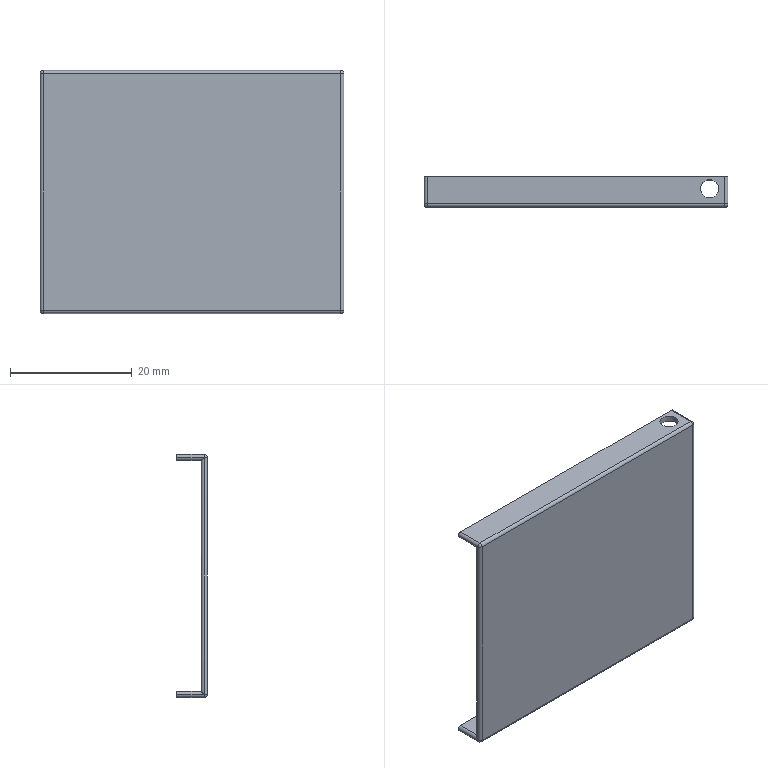Part | SolidWorks | features ICE 2, Extrusion 1, Fillet 1, MirrorPattern 1, MoveFace 1 | 1 solid | 31 faces | box 50 x 5 x 40 mm | volume 2370 mm3 | cylinder 19 | plane 8 | sphere 4 | commonest cylinder face diameters 1 x15 3 x4
STEP:
#1=CARTESIAN_POINT('',(23.5,3.,-19.));
#2=VERTEX_POINT('',#1);
#3=CARTESIAN_POINT('',(20.5,3.,-19.));
#4=VERTEX_POINT('',#3);
#5=CARTESIAN_POINT('',(22.,3.,-19.));
#6=DIRECTION('',(0.,0.,-1.));
#7=DIRECTION('',(-1.,0.,0.));
#8=AXIS2_PLACEMENT_3D('',#5,#6,#7);
#9=CIRCLE('',#8,1.5);
#10=EDGE_CURVE('',#2,#4,#9,.T.);
#11=ORIENTED_EDGE('',*,*,#10,.F.);
#12=CARTESIAN_POINT('',(23.5,3.,-20.));
#13=VERTEX_POINT('',#12);
#14=CARTESIAN_POINT('',(23.5,3.,20.));
#15=DIRECTION('',(0.,0.,-1.));
#16=VECTOR('',#15,1000.);
#17=LINE('',#14,#16);
#18=EDGE_CURVE('',#2,#13,#17,.T.);
#19=ORIENTED_EDGE('',*,*,#18,.T.);
#20=CARTESIAN_POINT('',(20.5,3.,-20.));
#21=VERTEX_POINT('',#20);
#22=CARTESIAN_POINT('',(22.,3.,-20.));
#23=DIRECTION('',(0.,0.,-1.));
#24=DIRECTION('',(-1.,0.,0.));
#25=AXIS2_PLACEMENT_3D('',#22,#23,#24);
#26=CIRCLE('',#25,1.5);
#27=EDGE_CURVE('',#13,#21,#26,.T.);
#28=ORIENTED_EDGE('',*,*,#27,.T.);
#29=CARTESIAN_POINT('',(20.5,3.,20.));
#30=DIRECTION('',(0.,0.,-1.));
#31=VECTOR('',#30,1000.);
#32=LINE('',#29,#31);
#33=EDGE_CURVE('',#4,#21,#32,.T.);
#34=ORIENTED_EDGE('',*,*,#33,.F.);
#35=EDGE_LOOP('',(#11,#19,#28,#34));
#36=FACE_OUTER_BOUND('',#35,.T.);
#37=CARTESIAN_POINT('',(22.,3.,20.));
#38=DIRECTION('',(0.,0.,-1.));
#39=DIRECTION('',(-1.,0.,0.));
#40=AXIS2_PLACEMENT_3D('',#37,#38,#39);
#41=CYLINDRICAL_SURFACE('',#40,1.5);
#42=ADVANCED_FACE('',(#36),#41,.F.);
#43=CARTESIAN_POINT('',(23.5,3.,20.));
#44=VERTEX_POINT('',#43);
#45=CARTESIAN_POINT('',(20.5,3.,20.));
#46=VERTEX_POINT('',#45);
#47=CARTESIAN_POINT('',(22.,3.,20.));
#48=DIRECTION('',(0.,0.,-1.));
#49=DIRECTION('',(-1.,0.,0.));
#50=AXIS2_PLACEMENT_3D('',#47,#48,#49);
#51=CIRCLE('',#50,1.5);
#52=EDGE_CURVE('',#44,#46,#51,.T.);
#53=ORIENTED_EDGE('',*,*,#52,.F.);
#54=CARTESIAN_POINT('',(23.5,3.,19.));
#55=VERTEX_POINT('',#54);
#56=CARTESIAN_POINT('',(23.5,3.,20.));
#57=DIRECTION('',(0.,0.,-1.));
#58=VECTOR('',#57,1000.);
#59=LINE('',#56,#58);
#60=EDGE_CURVE('',#44,#55,#59,.T.);
#61=ORIENTED_EDGE('',*,*,#60,.T.);
#62=CARTESIAN_POINT('',(20.5,3.,19.));
#63=VERTEX_POINT('',#62);
#64=CARTESIAN_POINT('',(22.,3.,19.));
#65=DIRECTION('',(0.,0.,1.));
#66=DIRECTION('',(1.,0.,0.));
#67=AXIS2_PLACEMENT_3D('',#64,#65,#66);
#68=CIRCLE('',#67,1.5);
#69=EDGE_CURVE('',#63,#55,#68,.T.);
#70=ORIENTED_EDGE('',*,*,#69,.F.);
#71=CARTESIAN_POINT('',(20.5,3.,20.));
#72=DIRECTION('',(0.,0.,-1.));
#73=VECTOR('',#72,1000.);
#74=LINE('',#71,#73);
#75=EDGE_CURVE('',#46,#63,#74,.T.);
#76=ORIENTED_EDGE('',*,*,#75,.F.);
#77=EDGE_LOOP('',(#53,#61,#70,#76));
#78=FACE_OUTER_BOUND('',#77,.T.);
#79=CARTESIAN_POINT('',(22.,3.,20.));
#80=DIRECTION('',(0.,0.,-1.));
#81=DIRECTION('',(-1.,0.,0.));
#82=AXIS2_PLACEMENT_3D('',#79,#80,#81);
#83=CYLINDRICAL_SURFACE('',#82,1.5);
#84=ADVANCED_FACE('',(#78),#83,.F.);
#85=CARTESIAN_POINT('',(24.5,1.,19.));
#86=VERTEX_POINT('',#85);
#87=CARTESIAN_POINT('',(-24.5,1.,19.));
#88=VERTEX_POINT('',#87);
#89=CARTESIAN_POINT('',(-25.,1.,19.));
#90=DIRECTION('',(-1.,0.,0.));
#91=VECTOR('',#90,1000.);
#92=LINE('',#89,#91);
#93=EDGE_CURVE('',#86,#88,#92,.T.);
#94=ORIENTED_EDGE('',*,*,#93,.F.);
#95=CARTESIAN_POINT('',(24.5,1.,-19.));
#96=VERTEX_POINT('',#95);
#97=CARTESIAN_POINT('',(24.5,1.,0.));
#98=DIRECTION('',(0.,0.,-1.));
#99=VECTOR('',#98,1000.);
#100=LINE('',#97,#99);
#101=EDGE_CURVE('',#86,#96,#100,.T.);
#102=ORIENTED_EDGE('',*,*,#101,.T.);
#103=CARTESIAN_POINT('',(-24.5,1.,-19.));
#104=VERTEX_POINT('',#103);
#105=CARTESIAN_POINT('',(-25.,1.,-19.));
#106=DIRECTION('',(-1.,0.,0.));
#107=VECTOR('',#106,1000.);
#108=LINE('',#105,#107);
#109=EDGE_CURVE('',#96,#104,#108,.T.);
#110=ORIENTED_EDGE('',*,*,#109,.T.);
#111=CARTESIAN_POINT('',(-24.5,1.,0.));
#112=DIRECTION('',(0.,0.,1.));
#113=VECTOR('',#112,1000.);
#114=LINE('',#111,#113);
#115=EDGE_CURVE('',#104,#88,#114,.T.);
#116=ORIENTED_EDGE('',*,*,#115,.T.);
#117=EDGE_LOOP('',(#94,#102,#110,#116));
#118=FACE_OUTER_BOUND('',#117,.T.);
#119=CARTESIAN_POINT('',(0.,1.,0.));
#120=DIRECTION('',(0.,-1.,0.));
#121=DIRECTION('',(0.,0.,-1.));
#122=AXIS2_PLACEMENT_3D('',#119,#120,#121);
#123=PLANE('',#122);
#124=ADVANCED_FACE('',(#118),#123,.F.);
#125=CARTESIAN_POINT('',(22.,3.,-20.));
#126=DIRECTION('',(0.,0.,-1.));
#127=DIRECTION('',(-1.,0.,0.));
#128=AXIS2_PLACEMENT_3D('',#125,#126,#127);
#129=CIRCLE('',#128,1.5);
#130=EDGE_CURVE('',#21,#13,#129,.T.);
#131=ORIENTED_EDGE('',*,*,#130,.F.);
#132=ORIENTED_EDGE('',*,*,#27,.F.);
#133=EDGE_LOOP('',(#131,#132));
#134=FACE_BOUND('',#133,.T.);
#135=CARTESIAN_POINT('',(24.5,0.5,-20.));
#136=VERTEX_POINT('',#135);
#137=CARTESIAN_POINT('',(-24.5,0.5,-20.));
#138=VERTEX_POINT('',#137);
#139=CARTESIAN_POINT('',(-25.,0.5,-20.));
#140=DIRECTION('',(-1.,0.,0.));
#141=VECTOR('',#140,1000.);
#142=LINE('',#139,#141);
#143=EDGE_CURVE('',#136,#138,#142,.T.);
#144=ORIENTED_EDGE('',*,*,#143,.T.);
#145=CARTESIAN_POINT('',(-24.5,5.,-20.));
#146=VERTEX_POINT('',#145);
#147=CARTESIAN_POINT('',(-24.5,1.,-20.));
#148=DIRECTION('',(0.,1.,0.));
#149=VECTOR('',#148,1000.);
#150=LINE('',#147,#149);
#151=EDGE_CURVE('',#138,#146,#150,.T.);
#152=ORIENTED_EDGE('',*,*,#151,.T.);
#153=CARTESIAN_POINT('',(24.5,5.,-20.));
#154=VERTEX_POINT('',#153);
#155=CARTESIAN_POINT('',(-25.,5.,-20.));
#156=DIRECTION('',(1.,0.,0.));
#157=VECTOR('',#156,1000.);
#158=LINE('',#155,#157);
#159=EDGE_CURVE('',#146,#154,#158,.T.);
#160=ORIENTED_EDGE('',*,*,#159,.T.);
#161=CARTESIAN_POINT('',(24.5,1.,-20.));
#162=DIRECTION('',(0.,-1.,0.));
#163=VECTOR('',#162,1000.);
#164=LINE('',#161,#163);
#165=EDGE_CURVE('',#154,#136,#164,.T.);
#166=ORIENTED_EDGE('',*,*,#165,.T.);
#167=EDGE_LOOP('',(#144,#152,#160,#166));
#168=FACE_OUTER_BOUND('',#167,.T.);
#169=CARTESIAN_POINT('',(-25.,1.,-20.));
#170=DIRECTION('',(0.,0.,1.));
#171=DIRECTION('',(1.,0.,0.));
#172=AXIS2_PLACEMENT_3D('',#169,#170,#171);
#173=PLANE('',#172);
#174=ADVANCED_FACE('',(#134,#168),#173,.F.);
#175=CARTESIAN_POINT('',(22.,3.,20.));
#176=DIRECTION('',(0.,0.,-1.));
#177=DIRECTION('',(-1.,0.,0.));
#178=AXIS2_PLACEMENT_3D('',#175,#176,#177);
#179=CIRCLE('',#178,1.5);
#180=EDGE_CURVE('',#46,#44,#179,.T.);
#181=ORIENTED_EDGE('',*,*,#180,.T.);
#182=ORIENTED_EDGE('',*,*,#52,.T.);
#183=EDGE_LOOP('',(#181,#182));
#184=FACE_BOUND('',#183,.T.);
#185=CARTESIAN_POINT('',(-24.5,5.,20.));
#186=VERTEX_POINT('',#185);
#187=CARTESIAN_POINT('',(24.5,5.,20.));
#188=VERTEX_POINT('',#187);
#189=CARTESIAN_POINT('',(-25.,5.,20.));
#190=DIRECTION('',(1.,0.,0.));
#191=VECTOR('',#190,1000.);
#192=LINE('',#189,#191);
#193=EDGE_CURVE('',#186,#188,#192,.T.);
#194=ORIENTED_EDGE('',*,*,#193,.F.);
#195=CARTESIAN_POINT('',(-24.5,0.5,20.));
#196=VERTEX_POINT('',#195);
#197=CARTESIAN_POINT('',(-24.5,1.,20.));
#198=DIRECTION('',(0.,-1.,0.));
#199=VECTOR('',#198,1000.);
#200=LINE('',#197,#199);
#201=EDGE_CURVE('',#186,#196,#200,.T.);
#202=ORIENTED_EDGE('',*,*,#201,.T.);
#203=CARTESIAN_POINT('',(24.5,0.5,20.));
#204=VERTEX_POINT('',#203);
#205=CARTESIAN_POINT('',(25.,0.5,20.));
#206=DIRECTION('',(1.,0.,0.));
#207=VECTOR('',#206,1000.);
#208=LINE('',#205,#207);
#209=EDGE_CURVE('',#196,#204,#208,.T.);
#210=ORIENTED_EDGE('',*,*,#209,.T.);
#211=CARTESIAN_POINT('',(24.5,1.,20.));
#212=DIRECTION('',(0.,1.,0.));
#213=VECTOR('',#212,1000.);
#214=LINE('',#211,#213);
#215=EDGE_CURVE('',#204,#188,#214,.T.);
#216=ORIENTED_EDGE('',*,*,#215,.T.);
#217=EDGE_LOOP('',(#194,#202,#210,#216));
#218=FACE_OUTER_BOUND('',#217,.T.);
#219=CARTESIAN_POINT('',(-25.,1.,20.));
#220=DIRECTION('',(0.,0.,-1.));
#221=DIRECTION('',(-1.,0.,0.));
#222=AXIS2_PLACEMENT_3D('',#219,#220,#221);
#223=PLANE('',#222);
#224=ADVANCED_FACE('',(#184,#218),#223,.F.);
#225=CARTESIAN_POINT('',(-24.5,0.,19.5));
#226=VERTEX_POINT('',#225);
#227=CARTESIAN_POINT('',(-24.5,0.,-19.5));
#228=VERTEX_POINT('',#227);
#229=CARTESIAN_POINT('',(-24.5,0.,-20.));
#230=DIRECTION('',(0.,0.,-1.));
#231=VECTOR('',#230,1000.);
#232=LINE('',#229,#231);
#233=EDGE_CURVE('',#226,#228,#232,.T.);
#234=ORIENTED_EDGE('',*,*,#233,.T.);
#235=CARTESIAN_POINT('',(24.5,0.,-19.5));
#236=VERTEX_POINT('',#235);
#237=CARTESIAN_POINT('',(25.,0.,-19.5));
#238=DIRECTION('',(1.,0.,0.));
#239=VECTOR('',#238,1000.);
#240=LINE('',#237,#239);
#241=EDGE_CURVE('',#228,#236,#240,.T.);
#242=ORIENTED_EDGE('',*,*,#241,.T.);
#243=CARTESIAN_POINT('',(24.5,0.,19.5));
#244=VERTEX_POINT('',#243);
#245=CARTESIAN_POINT('',(24.5,0.,20.));
#246=DIRECTION('',(0.,0.,1.));
#247=VECTOR('',#246,1000.);
#248=LINE('',#245,#247);
#249=EDGE_CURVE('',#236,#244,#248,.T.);
#250=ORIENTED_EDGE('',*,*,#249,.T.);
#251=CARTESIAN_POINT('',(-25.,0.,19.5));
#252=DIRECTION('',(-1.,0.,0.));
#253=VECTOR('',#252,1000.);
#254=LINE('',#251,#253);
#255=EDGE_CURVE('',#244,#226,#254,.T.);
#256=ORIENTED_EDGE('',*,*,#255,.T.);
#257=EDGE_LOOP('',(#234,#242,#250,#256));
#258=FACE_OUTER_BOUND('',#257,.T.);
#259=CARTESIAN_POINT('',(0.,0.,0.));
#260=DIRECTION('',(0.,-1.,0.));
#261=DIRECTION('',(0.,0.,-1.));
#262=AXIS2_PLACEMENT_3D('',#259,#260,#261);
#263=PLANE('',#262);
#264=ADVANCED_FACE('',(#258),#263,.T.);
#265=CARTESIAN_POINT('',(-25.,5.,-19.5));
#266=VERTEX_POINT('',#265);
#267=CARTESIAN_POINT('',(-24.5,5.,-19.5));
#268=DIRECTION('',(0.,1.,0.));
#269=DIRECTION('',(-1.,0.,0.));
#270=AXIS2_PLACEMENT_3D('',#267,#268,#269);
#271=CIRCLE('',#270,0.5);
#272=EDGE_CURVE('',#146,#266,#271,.T.);
#273=ORIENTED_EDGE('',*,*,#272,.T.);
#274=CARTESIAN_POINT('',(-24.5,5.,-19.));
#275=VERTEX_POINT('',#274);
#276=CARTESIAN_POINT('',(-24.5,5.,-19.5));
#277=DIRECTION('',(0.,1.,0.));
#278=DIRECTION('',(-1.,0.,0.));
#279=AXIS2_PLACEMENT_3D('',#276,#277,#278);
#280=CIRCLE('',#279,0.5);
#281=EDGE_CURVE('',#266,#275,#280,.T.);
#282=ORIENTED_EDGE('',*,*,#281,.T.);
#283=CARTESIAN_POINT('',(24.5,5.,-19.));
#284=VERTEX_POINT('',#283);
#285=CARTESIAN_POINT('',(-25.,5.,-19.));
#286=DIRECTION('',(1.,0.,0.));
#287=VECTOR('',#286,1000.);
#288=LINE('',#285,#287);
#289=EDGE_CURVE('',#275,#284,#288,.T.);
#290=ORIENTED_EDGE('',*,*,#289,.T.);
#291=CARTESIAN_POINT('',(24.5,5.,-20.));
#292=DIRECTION('',(0.,0.,-1.));
#293=VECTOR('',#292,1000.);
#294=LINE('',#291,#293);
#295=EDGE_CURVE('',#284,#154,#294,.T.);
#296=ORIENTED_EDGE('',*,*,#295,.T.);
#297=ORIENTED_EDGE('',*,*,#159,.F.);
#298=EDGE_LOOP('',(#273,#282,#290,#296,#297));
#299=FACE_OUTER_BOUND('',#298,.T.);
#300=CARTESIAN_POINT('',(-25.,5.,-19.));
#301=DIRECTION('',(0.,1.,0.));
#302=DIRECTION('',(-1.,0.,0.));
#303=AXIS2_PLACEMENT_3D('',#300,#301,#302);
#304=PLANE('',#303);
#305=ADVANCED_FACE('',(#299),#304,.T.);
#306=CARTESIAN_POINT('',(22.,3.,-19.));
#307=DIRECTION('',(0.,0.,-1.));
#308=DIRECTION('',(-1.,0.,0.));
#309=AXIS2_PLACEMENT_3D('',#306,#307,#308);
#310=CIRCLE('',#309,1.5);
#311=EDGE_CURVE('',#4,#2,#310,.T.);
#312=ORIENTED_EDGE('',*,*,#311,.T.);
#313=ORIENTED_EDGE('',*,*,#10,.T.);
#314=EDGE_LOOP('',(#312,#313));
#315=FACE_BOUND('',#314,.T.);
#316=ORIENTED_EDGE('',*,*,#109,.F.);
#317=CARTESIAN_POINT('',(24.5,0.,-19.));
#318=DIRECTION('',(0.,1.,0.));
#319=VECTOR('',#318,1000.);
#320=LINE('',#317,#319);
#321=EDGE_CURVE('',#96,#284,#320,.T.);
#322=ORIENTED_EDGE('',*,*,#321,.T.);
#323=ORIENTED_EDGE('',*,*,#289,.F.);
#324=CARTESIAN_POINT('',(-24.5,0.,-19.));
#325=DIRECTION('',(0.,-1.,0.));
#326=VECTOR('',#325,1000.);
#327=LINE('',#324,#326);
#328=EDGE_CURVE('',#275,#104,#327,.T.);
#329=ORIENTED_EDGE('',*,*,#328,.T.);
#330=EDGE_LOOP('',(#316,#322,#323,#329));
#331=FACE_OUTER_BOUND('',#330,.T.);
#332=CARTESIAN_POINT('',(0.,0.,-19.));
#333=DIRECTION('',(0.,0.,-1.));
#334=DIRECTION('',(-1.,0.,0.));
#335=AXIS2_PLACEMENT_3D('',#332,#333,#334);
#336=PLANE('',#335);
#337=ADVANCED_FACE('',(#315,#331),#336,.F.);
#338=CARTESIAN_POINT('',(-24.5,5.,19.));
#339=VERTEX_POINT('',#338);
#340=CARTESIAN_POINT('',(24.5,5.,19.));
#341=VERTEX_POINT('',#340);
#342=CARTESIAN_POINT('',(-25.,5.,19.));
#343=DIRECTION('',(1.,0.,0.));
#344=VECTOR('',#343,1000.);
#345=LINE('',#342,#344);
#346=EDGE_CURVE('',#339,#341,#345,.T.);
#347=ORIENTED_EDGE('',*,*,#346,.F.);
#348=CARTESIAN_POINT('',(-25.,5.,19.5));
#349=VERTEX_POINT('',#348);
#350=CARTESIAN_POINT('',(-24.5,5.,19.5));
#351=DIRECTION('',(0.,1.,0.));
#352=DIRECTION('',(1.,0.,0.));
#353=AXIS2_PLACEMENT_3D('',#350,#351,#352);
#354=CIRCLE('',#353,0.5);
#355=EDGE_CURVE('',#339,#349,#354,.T.);
#356=ORIENTED_EDGE('',*,*,#355,.T.);
#357=CARTESIAN_POINT('',(-24.5,5.,19.5));
#358=DIRECTION('',(0.,1.,0.));
#359=DIRECTION('',(1.,0.,0.));
#360=AXIS2_PLACEMENT_3D('',#357,#358,#359);
#361=CIRCLE('',#360,0.5);
#362=EDGE_CURVE('',#349,#186,#361,.T.);
#363=ORIENTED_EDGE('',*,*,#362,.T.);
#364=ORIENTED_EDGE('',*,*,#193,.T.);
#365=CARTESIAN_POINT('',(25.,5.,19.5));
#366=VERTEX_POINT('',#365);
#367=CARTESIAN_POINT('',(24.5,5.,19.5));
#368=DIRECTION('',(0.,1.,0.));
#369=DIRECTION('',(1.,0.,0.));
#370=AXIS2_PLACEMENT_3D('',#367,#368,#369);
#371=CIRCLE('',#370,0.5);
#372=EDGE_CURVE('',#188,#366,#371,.T.);
#373=ORIENTED_EDGE('',*,*,#372,.T.);
#374=CARTESIAN_POINT('',(24.5,5.,19.5));
#375=DIRECTION('',(0.,1.,0.));
#376=DIRECTION('',(1.,0.,0.));
#377=AXIS2_PLACEMENT_3D('',#374,#375,#376);
#378=CIRCLE('',#377,0.5);
#379=EDGE_CURVE('',#366,#341,#378,.T.);
#380=ORIENTED_EDGE('',*,*,#379,.T.);
#381=EDGE_LOOP('',(#347,#356,#363,#364,#373,#380));
#382=FACE_OUTER_BOUND('',#381,.T.);
#383=CARTESIAN_POINT('',(-25.,5.,19.));
#384=DIRECTION('',(0.,-1.,0.));
#385=DIRECTION('',(1.,0.,0.));
#386=AXIS2_PLACEMENT_3D('',#383,#384,#385);
#387=PLANE('',#386);
#388=ADVANCED_FACE('',(#382),#387,.F.);
#389=ORIENTED_EDGE('',*,*,#69,.T.);
#390=CARTESIAN_POINT('',(22.,3.,19.));
#391=DIRECTION('',(0.,0.,1.));
#392=DIRECTION('',(1.,0.,0.));
#393=AXIS2_PLACEMENT_3D('',#390,#391,#392);
#394=CIRCLE('',#393,1.5);
#395=EDGE_CURVE('',#55,#63,#394,.T.);
#396=ORIENTED_EDGE('',*,*,#395,.T.);
#397=EDGE_LOOP('',(#389,#396));
#398=FACE_BOUND('',#397,.T.);
#399=ORIENTED_EDGE('',*,*,#346,.T.);
#400=CARTESIAN_POINT('',(24.5,0.,19.));
#401=DIRECTION('',(0.,-1.,0.));
#402=VECTOR('',#401,1000.);
#403=LINE('',#400,#402);
#404=EDGE_CURVE('',#341,#86,#403,.T.);
#405=ORIENTED_EDGE('',*,*,#404,.T.);
#406=ORIENTED_EDGE('',*,*,#93,.T.);
#407=CARTESIAN_POINT('',(-24.5,0.,19.));
#408=DIRECTION('',(0.,1.,0.));
#409=VECTOR('',#408,1000.);
#410=LINE('',#407,#409);
#411=EDGE_CURVE('',#88,#339,#410,.T.);
#412=ORIENTED_EDGE('',*,*,#411,.T.);
#413=EDGE_LOOP('',(#399,#405,#406,#412));
#414=FACE_OUTER_BOUND('',#413,.T.);
#415=CARTESIAN_POINT('',(0.,0.,19.));
#416=DIRECTION('',(0.,0.,1.));
#417=DIRECTION('',(-1.,0.,0.));
#418=AXIS2_PLACEMENT_3D('',#415,#416,#417);
#419=PLANE('',#418);
#420=ADVANCED_FACE('',(#398,#414),#419,.F.);
#421=ORIENTED_EDGE('',*,*,#60,.F.);
#422=ORIENTED_EDGE('',*,*,#180,.F.);
#423=ORIENTED_EDGE('',*,*,#75,.T.);
#424=ORIENTED_EDGE('',*,*,#395,.F.);
#425=EDGE_LOOP('',(#421,#422,#423,#424));
#426=FACE_OUTER_BOUND('',#425,.T.);
#427=CARTESIAN_POINT('',(22.,3.,20.));
#428=DIRECTION('',(0.,0.,-1.));
#429=DIRECTION('',(-1.,0.,0.));
#430=AXIS2_PLACEMENT_3D('',#427,#428,#429);
#431=CYLINDRICAL_SURFACE('',#430,1.5);
#432=ADVANCED_FACE('',(#426),#431,.F.);
#433=ORIENTED_EDGE('',*,*,#18,.F.);
#434=ORIENTED_EDGE('',*,*,#311,.F.);
#435=ORIENTED_EDGE('',*,*,#33,.T.);
#436=ORIENTED_EDGE('',*,*,#130,.T.);
#437=EDGE_LOOP('',(#433,#434,#435,#436));
#438=FACE_OUTER_BOUND('',#437,.T.);
#439=CARTESIAN_POINT('',(22.,3.,20.));
#440=DIRECTION('',(0.,0.,-1.));
#441=DIRECTION('',(-1.,0.,0.));
#442=AXIS2_PLACEMENT_3D('',#439,#440,#441);
#443=CYLINDRICAL_SURFACE('',#442,1.5);
#444=ADVANCED_FACE('',(#438),#443,.F.);
#445=CARTESIAN_POINT('',(25.,0.5,19.5));
#446=VERTEX_POINT('',#445);
#447=CARTESIAN_POINT('',(25.,1.,19.5));
#448=DIRECTION('',(0.,-1.,0.));
#449=VECTOR('',#448,1000.);
#450=LINE('',#447,#449);
#451=EDGE_CURVE('',#366,#446,#450,.T.);
#452=ORIENTED_EDGE('',*,*,#451,.F.);
#453=ORIENTED_EDGE('',*,*,#372,.F.);
#454=ORIENTED_EDGE('',*,*,#215,.F.);
#455=CARTESIAN_POINT('',(24.5,0.5,19.5));
#456=DIRECTION('',(0.,-1.,0.));
#457=DIRECTION('',(0.,0.,-1.));
#458=AXIS2_PLACEMENT_3D('',#455,#456,#457);
#459=CIRCLE('',#458,0.5);
#460=EDGE_CURVE('',#446,#204,#459,.T.);
#461=ORIENTED_EDGE('',*,*,#460,.F.);
#462=EDGE_LOOP('',(#452,#453,#454,#461));
#463=FACE_OUTER_BOUND('',#462,.T.);
#464=CARTESIAN_POINT('',(24.5,1.,19.5));
#465=DIRECTION('',(0.,-1.,0.));
#466=DIRECTION('',(0.,0.,-1.));
#467=AXIS2_PLACEMENT_3D('',#464,#465,#466);
#468=CYLINDRICAL_SURFACE('',#467,0.5);
#469=ADVANCED_FACE('',(#463),#468,.T.);
#470=ORIENTED_EDGE('',*,*,#379,.F.);
#471=ORIENTED_EDGE('',*,*,#451,.T.);
#472=CARTESIAN_POINT('',(24.5,1.,19.));
#473=CARTESIAN_POINT('',(24.793,1.,19.));
#474=CARTESIAN_POINT('',(25.,0.7929,19.207));
#475=CARTESIAN_POINT('',(25.,0.5,19.5));
#476=(BOUNDED_CURVE()B_SPLINE_CURVE(3,(#472,#473,#474,#475),.UNSPECIFIED.,.F.,.T.)B_SPLINE_CURVE_WITH_KNOTS((4,4),(0.,1.571),.UNSPECIFIED.)CURVE()GEOMETRIC_REPRESENTATION_ITEM()RATIONAL_B_SPLINE_CURVE((1.,0.8047,0.8047,1.))REPRESENTATION_ITEM(''));
#477=EDGE_CURVE('',#86,#446,#476,.T.);
#478=ORIENTED_EDGE('',*,*,#477,.F.);
#479=ORIENTED_EDGE('',*,*,#404,.F.);
#480=EDGE_LOOP('',(#470,#471,#478,#479));
#481=FACE_OUTER_BOUND('',#480,.T.);
#482=CARTESIAN_POINT('',(24.5,0.,19.5));
#483=DIRECTION('',(0.,-1.,0.));
#484=DIRECTION('',(0.,0.,-1.));
#485=AXIS2_PLACEMENT_3D('',#482,#483,#484);
#486=CYLINDRICAL_SURFACE('',#485,0.5);
#487=ADVANCED_FACE('',(#481),#486,.T.);
#488=CARTESIAN_POINT('',(-25.,0.5,19.5));
#489=VERTEX_POINT('',#488);
#490=CARTESIAN_POINT('',(-25.,1.,19.5));
#491=DIRECTION('',(0.,-1.,0.));
#492=VECTOR('',#491,1000.);
#493=LINE('',#490,#492);
#494=EDGE_CURVE('',#349,#489,#493,.T.);
#495=ORIENTED_EDGE('',*,*,#494,.F.);
#496=ORIENTED_EDGE('',*,*,#355,.F.);
#497=ORIENTED_EDGE('',*,*,#411,.F.);
#498=CARTESIAN_POINT('',(-25.,0.5,19.5));
#499=CARTESIAN_POINT('',(-25.,0.7929,19.207));
#500=CARTESIAN_POINT('',(-24.793,1.,19.));
#501=CARTESIAN_POINT('',(-24.5,1.,19.));
#502=(BOUNDED_CURVE()B_SPLINE_CURVE(3,(#498,#499,#500,#501),.UNSPECIFIED.,.F.,.T.)B_SPLINE_CURVE_WITH_KNOTS((4,4),(1.571,3.142),.UNSPECIFIED.)CURVE()GEOMETRIC_REPRESENTATION_ITEM()RATIONAL_B_SPLINE_CURVE((1.,0.8047,0.8047,1.))REPRESENTATION_ITEM(''));
#503=EDGE_CURVE('',#489,#88,#502,.T.);
#504=ORIENTED_EDGE('',*,*,#503,.F.);
#505=EDGE_LOOP('',(#495,#496,#497,#504));
#506=FACE_OUTER_BOUND('',#505,.T.);
#507=CARTESIAN_POINT('',(-24.5,0.,19.5));
#508=DIRECTION('',(0.,1.,0.));
#509=DIRECTION('',(0.,0.,1.));
#510=AXIS2_PLACEMENT_3D('',#507,#508,#509);
#511=CYLINDRICAL_SURFACE('',#510,0.5);
#512=ADVANCED_FACE('',(#506),#511,.T.);
#513=ORIENTED_EDGE('',*,*,#362,.F.);
#514=ORIENTED_EDGE('',*,*,#494,.T.);
#515=CARTESIAN_POINT('',(-24.5,0.5,19.5));
#516=DIRECTION('',(0.,-1.,0.));
#517=DIRECTION('',(0.,0.,-1.));
#518=AXIS2_PLACEMENT_3D('',#515,#516,#517);
#519=CIRCLE('',#518,0.5);
#520=EDGE_CURVE('',#196,#489,#519,.T.);
#521=ORIENTED_EDGE('',*,*,#520,.F.);
#522=ORIENTED_EDGE('',*,*,#201,.F.);
#523=EDGE_LOOP('',(#513,#514,#521,#522));
#524=FACE_OUTER_BOUND('',#523,.T.);
#525=CARTESIAN_POINT('',(-24.5,1.,19.5));
#526=DIRECTION('',(0.,-1.,0.));
#527=DIRECTION('',(0.,0.,-1.));
#528=AXIS2_PLACEMENT_3D('',#525,#526,#527);
#529=CYLINDRICAL_SURFACE('',#528,0.5);
#530=ADVANCED_FACE('',(#524),#529,.T.);
#531=CARTESIAN_POINT('',(24.5,0.5,19.5));
#532=DIRECTION('',(1.,0.,0.));
#533=DIRECTION('',(0.,0.,-1.));
#534=AXIS2_PLACEMENT_3D('',#531,#532,#533);
#535=CIRCLE('',#534,0.5);
#536=EDGE_CURVE('',#204,#244,#535,.T.);
#537=ORIENTED_EDGE('',*,*,#536,.F.);
#538=ORIENTED_EDGE('',*,*,#209,.F.);
#539=CARTESIAN_POINT('',(-24.5,0.5,19.5));
#540=DIRECTION('',(-1.,0.,0.));
#541=DIRECTION('',(0.,0.,1.));
#542=AXIS2_PLACEMENT_3D('',#539,#540,#541);
#543=CIRCLE('',#542,0.5);
#544=EDGE_CURVE('',#226,#196,#543,.T.);
#545=ORIENTED_EDGE('',*,*,#544,.F.);
#546=ORIENTED_EDGE('',*,*,#255,.F.);
#547=EDGE_LOOP('',(#537,#538,#545,#546));
#548=FACE_OUTER_BOUND('',#547,.T.);
#549=CARTESIAN_POINT('',(-25.,0.5,19.5));
#550=DIRECTION('',(-1.,0.,0.));
#551=DIRECTION('',(0.,0.,1.));
#552=AXIS2_PLACEMENT_3D('',#549,#550,#551);
#553=CYLINDRICAL_SURFACE('',#552,0.5);
#554=ADVANCED_FACE('',(#548),#553,.T.);
#555=ORIENTED_EDGE('',*,*,#460,.T.);
#556=ORIENTED_EDGE('',*,*,#536,.T.);
#557=CARTESIAN_POINT('',(24.5,0.5,19.5));
#558=DIRECTION('',(0.,0.,-1.));
#559=DIRECTION('',(1.,0.,0.));
#560=AXIS2_PLACEMENT_3D('',#557,#558,#559);
#561=CIRCLE('',#560,0.5);
#562=EDGE_CURVE('',#446,#244,#561,.T.);
#563=ORIENTED_EDGE('',*,*,#562,.F.);
#564=EDGE_LOOP('',(#555,#556,#563));
#565=FACE_OUTER_BOUND('',#564,.T.);
#566=CARTESIAN_POINT('',(24.5,0.5,19.5));
#567=DIRECTION('',(0.,1.,0.));
#568=DIRECTION('',(1.,0.,0.));
#569=AXIS2_PLACEMENT_3D('',#566,#567,#568);
#570=SPHERICAL_SURFACE('',#569,0.5);
#571=ADVANCED_FACE('',(#565),#570,.T.);
#572=CARTESIAN_POINT('',(25.,0.5,-19.5));
#573=VERTEX_POINT('',#572);
#574=CARTESIAN_POINT('',(24.5,1.,-19.));
#575=CARTESIAN_POINT('',(24.793,1.,-19.));
#576=CARTESIAN_POINT('',(25.,0.7929,-19.207));
#577=CARTESIAN_POINT('',(25.,0.5,-19.5));
#578=(BOUNDED_CURVE()B_SPLINE_CURVE(3,(#574,#575,#576,#577),.UNSPECIFIED.,.F.,.T.)B_SPLINE_CURVE_WITH_KNOTS((4,4),(3.142,4.712),.UNSPECIFIED.)CURVE()GEOMETRIC_REPRESENTATION_ITEM()RATIONAL_B_SPLINE_CURVE((1.,0.8047,0.8047,1.))REPRESENTATION_ITEM(''));
#579=EDGE_CURVE('',#96,#573,#578,.T.);
#580=ORIENTED_EDGE('',*,*,#579,.F.);
#581=ORIENTED_EDGE('',*,*,#101,.F.);
#582=ORIENTED_EDGE('',*,*,#477,.T.);
#583=CARTESIAN_POINT('',(25.,0.5,20.));
#584=DIRECTION('',(0.,0.,1.));
#585=VECTOR('',#584,1000.);
#586=LINE('',#583,#585);
#587=EDGE_CURVE('',#573,#446,#586,.T.);
#588=ORIENTED_EDGE('',*,*,#587,.F.);
#589=EDGE_LOOP('',(#580,#581,#582,#588));
#590=FACE_OUTER_BOUND('',#589,.T.);
#591=CARTESIAN_POINT('',(24.5,0.5,0.));
#592=DIRECTION('',(0.,0.,-1.));
#593=DIRECTION('',(-1.,0.,0.));
#594=AXIS2_PLACEMENT_3D('',#591,#592,#593);
#595=CYLINDRICAL_SURFACE('',#594,0.5);
#596=ADVANCED_FACE('',(#590),#595,.T.);
#597=CARTESIAN_POINT('',(25.,4.5,-19.5));
#598=VERTEX_POINT('',#597);
#599=CARTESIAN_POINT('',(24.5,5.,-19.));
#600=CARTESIAN_POINT('',(24.793,5.,-19.));
#601=CARTESIAN_POINT('',(25.,4.793,-19.207));
#602=CARTESIAN_POINT('',(25.,4.5,-19.5));
#603=(BOUNDED_CURVE()B_SPLINE_CURVE(3,(#599,#600,#601,#602),.UNSPECIFIED.,.F.,.T.)B_SPLINE_CURVE_WITH_KNOTS((4,4),(0.,1.571),.UNSPECIFIED.)CURVE()GEOMETRIC_REPRESENTATION_ITEM()RATIONAL_B_SPLINE_CURVE((1.,0.8047,0.8047,1.))REPRESENTATION_ITEM(''));
#604=EDGE_CURVE('',#284,#598,#603,.T.);
#605=ORIENTED_EDGE('',*,*,#604,.F.);
#606=ORIENTED_EDGE('',*,*,#321,.F.);
#607=ORIENTED_EDGE('',*,*,#579,.T.);
#608=CARTESIAN_POINT('',(25.,1.,-19.5));
#609=DIRECTION('',(0.,-1.,0.));
#610=VECTOR('',#609,1000.);
#611=LINE('',#608,#610);
#612=EDGE_CURVE('',#598,#573,#611,.T.);
#613=ORIENTED_EDGE('',*,*,#612,.F.);
#614=EDGE_LOOP('',(#605,#606,#607,#613));
#615=FACE_OUTER_BOUND('',#614,.T.);
#616=CARTESIAN_POINT('',(24.5,1.,-19.5));
#617=DIRECTION('',(0.,-1.,0.));
#618=DIRECTION('',(0.,0.,-1.));
#619=AXIS2_PLACEMENT_3D('',#616,#617,#618);
#620=CYLINDRICAL_SURFACE('',#619,0.5);
#621=ADVANCED_FACE('',(#615),#620,.T.);
#622=ORIENTED_EDGE('',*,*,#295,.F.);
#623=ORIENTED_EDGE('',*,*,#604,.T.);
#624=CARTESIAN_POINT('',(24.5,5.,-20.));
#625=CARTESIAN_POINT('',(24.793,5.,-20.));
#626=CARTESIAN_POINT('',(25.,4.793,-19.793));
#627=CARTESIAN_POINT('',(25.,4.5,-19.5));
#628=(BOUNDED_CURVE()B_SPLINE_CURVE(3,(#624,#625,#626,#627),.UNSPECIFIED.,.F.,.F.)B_SPLINE_CURVE_WITH_KNOTS((4,4),(3.142,4.712),.UNSPECIFIED.)CURVE()GEOMETRIC_REPRESENTATION_ITEM()RATIONAL_B_SPLINE_CURVE((1.,0.8047,0.8047,1.))REPRESENTATION_ITEM(''));
#629=EDGE_CURVE('',#154,#598,#628,.T.);
#630=ORIENTED_EDGE('',*,*,#629,.F.);
#631=EDGE_LOOP('',(#622,#623,#630));
#632=FACE_OUTER_BOUND('',#631,.T.);
#633=CARTESIAN_POINT('',(24.5,4.5,-19.));
#634=DIRECTION('',(0.,0.,1.));
#635=DIRECTION('',(1.,0.,0.));
#636=AXIS2_PLACEMENT_3D('',#633,#634,#635);
#637=CYLINDRICAL_SURFACE('',#636,0.5);
#638=ADVANCED_FACE('',(#632),#637,.T.);
#639=CARTESIAN_POINT('',(-25.,0.5,-19.5));
#640=VERTEX_POINT('',#639);
#641=CARTESIAN_POINT('',(-24.5,1.,-19.));
#642=CARTESIAN_POINT('',(-24.793,1.,-19.));
#643=CARTESIAN_POINT('',(-25.,0.7929,-19.207));
#644=CARTESIAN_POINT('',(-25.,0.5,-19.5));
#645=(BOUNDED_CURVE()B_SPLINE_CURVE(3,(#641,#642,#643,#644),.UNSPECIFIED.,.F.,.F.)B_SPLINE_CURVE_WITH_KNOTS((4,4),(0.,1.571),.UNSPECIFIED.)CURVE()GEOMETRIC_REPRESENTATION_ITEM()RATIONAL_B_SPLINE_CURVE((1.,0.8047,0.8047,1.))REPRESENTATION_ITEM(''));
#646=EDGE_CURVE('',#104,#640,#645,.T.);
#647=ORIENTED_EDGE('',*,*,#646,.F.);
#648=ORIENTED_EDGE('',*,*,#328,.F.);
#649=ORIENTED_EDGE('',*,*,#281,.F.);
#650=CARTESIAN_POINT('',(-25.,1.,-19.5));
#651=DIRECTION('',(0.,1.,0.));
#652=VECTOR('',#651,1000.);
#653=LINE('',#650,#652);
#654=EDGE_CURVE('',#640,#266,#653,.T.);
#655=ORIENTED_EDGE('',*,*,#654,.F.);
#656=EDGE_LOOP('',(#647,#648,#649,#655));
#657=FACE_OUTER_BOUND('',#656,.T.);
#658=CARTESIAN_POINT('',(-24.5,1.,-19.5));
#659=DIRECTION('',(0.,1.,0.));
#660=DIRECTION('',(0.,0.,1.));
#661=AXIS2_PLACEMENT_3D('',#658,#659,#660);
#662=CYLINDRICAL_SURFACE('',#661,0.5);
#663=ADVANCED_FACE('',(#657),#662,.T.);
#664=ORIENTED_EDGE('',*,*,#115,.F.);
#665=ORIENTED_EDGE('',*,*,#646,.T.);
#666=CARTESIAN_POINT('',(-25.,0.5,20.));
#667=DIRECTION('',(0.,0.,-1.));
#668=VECTOR('',#667,1000.);
#669=LINE('',#666,#668);
#670=EDGE_CURVE('',#489,#640,#669,.T.);
#671=ORIENTED_EDGE('',*,*,#670,.F.);
#672=ORIENTED_EDGE('',*,*,#503,.T.);
#673=EDGE_LOOP('',(#664,#665,#671,#672));
#674=FACE_OUTER_BOUND('',#673,.T.);
#675=CARTESIAN_POINT('',(-24.5,0.5,0.));
#676=DIRECTION('',(0.,0.,1.));
#677=DIRECTION('',(1.,0.,0.));
#678=AXIS2_PLACEMENT_3D('',#675,#676,#677);
#679=CYLINDRICAL_SURFACE('',#678,0.5);
#680=ADVANCED_FACE('',(#674),#679,.T.);
#681=ORIENTED_EDGE('',*,*,#544,.T.);
#682=ORIENTED_EDGE('',*,*,#520,.T.);
#683=CARTESIAN_POINT('',(-24.5,0.5,19.5));
#684=DIRECTION('',(0.,0.,-1.));
#685=DIRECTION('',(1.,0.,0.));
#686=AXIS2_PLACEMENT_3D('',#683,#684,#685);
#687=CIRCLE('',#686,0.5);
#688=EDGE_CURVE('',#226,#489,#687,.T.);
#689=ORIENTED_EDGE('',*,*,#688,.F.);
#690=EDGE_LOOP('',(#681,#682,#689));
#691=FACE_OUTER_BOUND('',#690,.T.);
#692=CARTESIAN_POINT('',(-24.5,0.5,19.5));
#693=DIRECTION('',(0.,1.,0.));
#694=DIRECTION('',(1.,0.,0.));
#695=AXIS2_PLACEMENT_3D('',#692,#693,#694);
#696=SPHERICAL_SURFACE('',#695,0.5);
#697=ADVANCED_FACE('',(#691),#696,.T.);
#698=ORIENTED_EDGE('',*,*,#562,.T.);
#699=ORIENTED_EDGE('',*,*,#249,.F.);
#700=CARTESIAN_POINT('',(24.5,0.5,-19.5));
#701=DIRECTION('',(0.,0.,-1.));
#702=DIRECTION('',(-1.,0.,0.));
#703=AXIS2_PLACEMENT_3D('',#700,#701,#702);
#704=CIRCLE('',#703,0.5);
#705=EDGE_CURVE('',#573,#236,#704,.T.);
#706=ORIENTED_EDGE('',*,*,#705,.F.);
#707=ORIENTED_EDGE('',*,*,#587,.T.);
#708=EDGE_LOOP('',(#698,#699,#706,#707));
#709=FACE_OUTER_BOUND('',#708,.T.);
#710=CARTESIAN_POINT('',(24.5,0.5,20.));
#711=DIRECTION('',(0.,0.,1.));
#712=DIRECTION('',(1.,0.,0.));
#713=AXIS2_PLACEMENT_3D('',#710,#711,#712);
#714=CYLINDRICAL_SURFACE('',#713,0.5);
#715=ADVANCED_FACE('',(#709),#714,.T.);
#716=ORIENTED_EDGE('',*,*,#629,.T.);
#717=ORIENTED_EDGE('',*,*,#612,.T.);
#718=CARTESIAN_POINT('',(24.5,0.5,-19.5));
#719=DIRECTION('',(0.,-1.,0.));
#720=DIRECTION('',(0.,0.,-1.));
#721=AXIS2_PLACEMENT_3D('',#718,#719,#720);
#722=CIRCLE('',#721,0.5);
#723=EDGE_CURVE('',#136,#573,#722,.T.);
#724=ORIENTED_EDGE('',*,*,#723,.F.);
#725=ORIENTED_EDGE('',*,*,#165,.F.);
#726=EDGE_LOOP('',(#716,#717,#724,#725));
#727=FACE_OUTER_BOUND('',#726,.T.);
#728=CARTESIAN_POINT('',(24.5,1.,-19.5));
#729=DIRECTION('',(0.,-1.,0.));
#730=DIRECTION('',(0.,0.,-1.));
#731=AXIS2_PLACEMENT_3D('',#728,#729,#730);
#732=CYLINDRICAL_SURFACE('',#731,0.5);
#733=ADVANCED_FACE('',(#727),#732,.T.);
#734=ORIENTED_EDGE('',*,*,#272,.F.);
#735=ORIENTED_EDGE('',*,*,#151,.F.);
#736=CARTESIAN_POINT('',(-24.5,0.5,-19.5));
#737=DIRECTION('',(0.,-1.,0.));
#738=DIRECTION('',(0.,0.,-1.));
#739=AXIS2_PLACEMENT_3D('',#736,#737,#738);
#740=CIRCLE('',#739,0.5);
#741=EDGE_CURVE('',#640,#138,#740,.T.);
#742=ORIENTED_EDGE('',*,*,#741,.F.);
#743=ORIENTED_EDGE('',*,*,#654,.T.);
#744=EDGE_LOOP('',(#734,#735,#742,#743));
#745=FACE_OUTER_BOUND('',#744,.T.);
#746=CARTESIAN_POINT('',(-24.5,1.,-19.5));
#747=DIRECTION('',(0.,-1.,0.));
#748=DIRECTION('',(0.,0.,-1.));
#749=AXIS2_PLACEMENT_3D('',#746,#747,#748);
#750=CYLINDRICAL_SURFACE('',#749,0.5);
#751=ADVANCED_FACE('',(#745),#750,.T.);
#752=ORIENTED_EDGE('',*,*,#688,.T.);
#753=ORIENTED_EDGE('',*,*,#670,.T.);
#754=CARTESIAN_POINT('',(-24.5,0.5,-19.5));
#755=DIRECTION('',(0.,0.,-1.));
#756=DIRECTION('',(-1.,0.,0.));
#757=AXIS2_PLACEMENT_3D('',#754,#755,#756);
#758=CIRCLE('',#757,0.5);
#759=EDGE_CURVE('',#228,#640,#758,.T.);
#760=ORIENTED_EDGE('',*,*,#759,.F.);
#761=ORIENTED_EDGE('',*,*,#233,.F.);
#762=EDGE_LOOP('',(#752,#753,#760,#761));
#763=FACE_OUTER_BOUND('',#762,.T.);
#764=CARTESIAN_POINT('',(-24.5,0.5,20.));
#765=DIRECTION('',(0.,0.,-1.));
#766=DIRECTION('',(-1.,0.,0.));
#767=AXIS2_PLACEMENT_3D('',#764,#765,#766);
#768=CYLINDRICAL_SURFACE('',#767,0.5);
#769=ADVANCED_FACE('',(#763),#768,.T.);
#770=ORIENTED_EDGE('',*,*,#723,.T.);
#771=ORIENTED_EDGE('',*,*,#705,.T.);
#772=CARTESIAN_POINT('',(24.5,0.5,-19.5));
#773=DIRECTION('',(-1.,0.,0.));
#774=DIRECTION('',(0.,0.,-1.));
#775=AXIS2_PLACEMENT_3D('',#772,#773,#774);
#776=CIRCLE('',#775,0.5);
#777=EDGE_CURVE('',#136,#236,#776,.T.);
#778=ORIENTED_EDGE('',*,*,#777,.F.);
#779=EDGE_LOOP('',(#770,#771,#778));
#780=FACE_OUTER_BOUND('',#779,.T.);
#781=CARTESIAN_POINT('',(24.5,0.5,-19.5));
#782=DIRECTION('',(0.,1.,0.));
#783=DIRECTION('',(1.,0.,0.));
#784=AXIS2_PLACEMENT_3D('',#781,#782,#783);
#785=SPHERICAL_SURFACE('',#784,0.5);
#786=ADVANCED_FACE('',(#780),#785,.T.);
#787=ORIENTED_EDGE('',*,*,#759,.T.);
#788=ORIENTED_EDGE('',*,*,#741,.T.);
#789=CARTESIAN_POINT('',(-24.5,0.5,-19.5));
#790=DIRECTION('',(1.,0.,0.));
#791=DIRECTION('',(0.,0.,1.));
#792=AXIS2_PLACEMENT_3D('',#789,#790,#791);
#793=CIRCLE('',#792,0.5);
#794=EDGE_CURVE('',#228,#138,#793,.T.);
#795=ORIENTED_EDGE('',*,*,#794,.F.);
#796=EDGE_LOOP('',(#787,#788,#795));
#797=FACE_OUTER_BOUND('',#796,.T.);
#798=CARTESIAN_POINT('',(-24.5,0.5,-19.5));
#799=DIRECTION('',(0.,1.,0.));
#800=DIRECTION('',(1.,0.,0.));
#801=AXIS2_PLACEMENT_3D('',#798,#799,#800);
#802=SPHERICAL_SURFACE('',#801,0.5);
#803=ADVANCED_FACE('',(#797),#802,.T.);
#804=ORIENTED_EDGE('',*,*,#777,.T.);
#805=ORIENTED_EDGE('',*,*,#241,.F.);
#806=ORIENTED_EDGE('',*,*,#794,.T.);
#807=ORIENTED_EDGE('',*,*,#143,.F.);
#808=EDGE_LOOP('',(#804,#805,#806,#807));
#809=FACE_OUTER_BOUND('',#808,.T.);
#810=CARTESIAN_POINT('',(-25.,0.5,-19.5));
#811=DIRECTION('',(1.,0.,0.));
#812=DIRECTION('',(0.,0.,-1.));
#813=AXIS2_PLACEMENT_3D('',#810,#811,#812);
#814=CYLINDRICAL_SURFACE('',#813,0.5);
#815=ADVANCED_FACE('',(#809),#814,.T.);
#816=CLOSED_SHELL('',(#42,#84,#124,#174,#224,#264,#305,#337,#388,#420,#432,#444,#469,#487,#512,#530,#554,#571,#596,#621,#638,#663,#680,#697,#715,#733,#751,#769,#786,#803,#815));
#817=MANIFOLD_SOLID_BREP('',#816);
#818=CARTESIAN_POINT('',(0.,0.,0.));
#819=DIRECTION('',(0.,0.,1.));
#820=DIRECTION('',(1.,0.,0.));
#821=AXIS2_PLACEMENT_3D('',#818,#819,#820);
#822=(LENGTH_UNIT()NAMED_UNIT(*)SI_UNIT(.MILLI.,.METRE.));
#823=UNCERTAINTY_MEASURE_WITH_UNIT(LENGTH_MEASURE(0.00001),#822,'','');
#824=(NAMED_UNIT(*)PLANE_ANGLE_UNIT()SI_UNIT($,.RADIAN.));
#825=(NAMED_UNIT(*)SI_UNIT($,.STERADIAN.)SOLID_ANGLE_UNIT());
#826=(GEOMETRIC_REPRESENTATION_CONTEXT(3)GLOBAL_UNCERTAINTY_ASSIGNED_CONTEXT((#823))GLOBAL_UNIT_ASSIGNED_CONTEXT((#822,#824,#825))REPRESENTATION_CONTEXT('',''));
#827=ADVANCED_BREP_SHAPE_REPRESENTATION('',(#817,#821),#826);